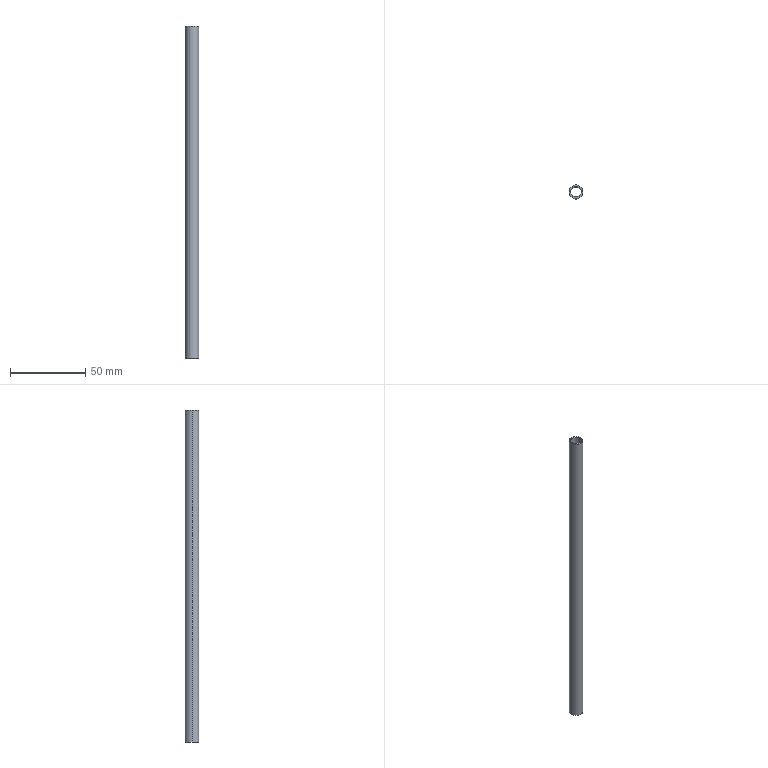Part | STEP file | DCV-000-018 | 1 solid | 6 faces | box 9 x 9 x 220 mm | volume 5529 mm3 | cylinder 4 | plane 2 | commonest cylinder face diameters 7 x2 9 x2
STEP:
#1=CARTESIAN_POINT('',(0.,0.,0.));
#2=DIRECTION('',(0.,0.,1.));
#3=DIRECTION('',(1.,0.,0.));
#4=AXIS2_PLACEMENT_3D('',#1,#2,#3);
#5=CARTESIAN_POINT('',(-3.5,0.,0.));
#6=VERTEX_POINT('',#5);
#7=CARTESIAN_POINT('',(-3.5,0.,220.));
#8=VERTEX_POINT('',#7);
#9=CARTESIAN_POINT('',(-3.5,0.,0.));
#10=DIRECTION('',(0.,0.,1.));
#11=VECTOR('',#10,1.);
#12=LINE('',#9,#11);
#13=CARTESIAN_POINT('',(0.,0.,0.));
#14=DIRECTION('',(0.,0.,1.));
#15=DIRECTION('',(-1.,0.,0.));
#16=AXIS2_PLACEMENT_3D('',#13,#14,#15);
#17=CYLINDRICAL_SURFACE('',#16,3.5);
#18=CARTESIAN_POINT('',(6.283,0.));
#19=DIRECTION('',(0.,1.));
#20=VECTOR('',#19,1.);
#21=LINE('',#18,#20);
#22=(GEOMETRIC_REPRESENTATION_CONTEXT(2)PARAMETRIC_REPRESENTATION_CONTEXT()REPRESENTATION_CONTEXT('',''));
#23=DEFINITIONAL_REPRESENTATION('',(#21),#22);
#24=PCURVE('',#17,#23);
#25=CARTESIAN_POINT('',(0.,0.,0.));
#26=DIRECTION('',(0.,0.,1.));
#27=DIRECTION('',(-1.,0.,0.));
#28=AXIS2_PLACEMENT_3D('',#25,#26,#27);
#29=CYLINDRICAL_SURFACE('',#28,3.5);
#30=CARTESIAN_POINT('',(0.,0.));
#31=DIRECTION('',(0.,1.));
#32=VECTOR('',#31,1.);
#33=LINE('',#30,#32);
#34=(GEOMETRIC_REPRESENTATION_CONTEXT(2)PARAMETRIC_REPRESENTATION_CONTEXT()REPRESENTATION_CONTEXT('',''));
#35=DEFINITIONAL_REPRESENTATION('',(#33),#34);
#36=PCURVE('',#29,#35);
#37=SURFACE_CURVE('',#12,(#24,#36),.PCURVE_S1.);
#38=EDGE_CURVE('',#6,#8,#37,.T.);
#39=ORIENTED_EDGE('',*,*,#38,.T.);
#40=CARTESIAN_POINT('',(3.5,0.,220.));
#41=VERTEX_POINT('',#40);
#42=CARTESIAN_POINT('',(0.,0.,220.));
#43=DIRECTION('',(0.,0.,-1.));
#44=DIRECTION('',(-1.,0.,0.));
#45=AXIS2_PLACEMENT_3D('',#42,#43,#44);
#46=CIRCLE('',#45,3.5);
#47=CARTESIAN_POINT('',(6.283,220.));
#48=DIRECTION('',(-1.,0.));
#49=VECTOR('',#48,1.);
#50=LINE('',#47,#49);
#51=(GEOMETRIC_REPRESENTATION_CONTEXT(2)PARAMETRIC_REPRESENTATION_CONTEXT()REPRESENTATION_CONTEXT('',''));
#52=DEFINITIONAL_REPRESENTATION('',(#50),#51);
#53=PCURVE('',#17,#52);
#54=CARTESIAN_POINT('',(0.,0.,220.));
#55=DIRECTION('',(0.,0.,1.));
#56=DIRECTION('',(1.,0.,0.));
#57=AXIS2_PLACEMENT_3D('',#54,#55,#56);
#58=PLANE('',#57);
#59=CARTESIAN_POINT('',(-3.5,0.));
#60=CARTESIAN_POINT('',(-3.5,6.062));
#61=CARTESIAN_POINT('',(1.75,3.031));
#62=CARTESIAN_POINT('',(7.,0.));
#63=CARTESIAN_POINT('',(1.75,-3.031));
#64=CARTESIAN_POINT('',(-3.5,-6.062));
#65=CARTESIAN_POINT('',(-3.5,0.));
#66=(BOUNDED_CURVE()B_SPLINE_CURVE(2,(#59,#60,#61,#62,#63,#64,#65),.UNSPECIFIED.,.T.,.F.)B_SPLINE_CURVE_WITH_KNOTS((1,2,2,2,2,1),(-2.094,0.,2.094,4.189,6.283,8.378),.UNSPECIFIED.)CURVE()GEOMETRIC_REPRESENTATION_ITEM()RATIONAL_B_SPLINE_CURVE((1.,0.5,1.,0.5,1.,0.5,1.))REPRESENTATION_ITEM(''));
#67=(GEOMETRIC_REPRESENTATION_CONTEXT(2)PARAMETRIC_REPRESENTATION_CONTEXT()REPRESENTATION_CONTEXT('',''));
#68=DEFINITIONAL_REPRESENTATION('',(#66),#67);
#69=PCURVE('',#58,#68);
#70=SURFACE_CURVE('',#46,(#53,#69),.PCURVE_S1.);
#71=EDGE_CURVE('',#8,#41,#70,.T.);
#72=ORIENTED_EDGE('',*,*,#71,.T.);
#73=CARTESIAN_POINT('',(3.5,0.,0.));
#74=VERTEX_POINT('',#73);
#75=CARTESIAN_POINT('',(3.5,0.,0.));
#76=DIRECTION('',(0.,0.,1.));
#77=VECTOR('',#76,1.);
#78=LINE('',#75,#77);
#79=CARTESIAN_POINT('',(3.142,0.));
#80=DIRECTION('',(0.,1.));
#81=VECTOR('',#80,1.);
#82=LINE('',#79,#81);
#83=(GEOMETRIC_REPRESENTATION_CONTEXT(2)PARAMETRIC_REPRESENTATION_CONTEXT()REPRESENTATION_CONTEXT('',''));
#84=DEFINITIONAL_REPRESENTATION('',(#82),#83);
#85=PCURVE('',#17,#84);
#86=CARTESIAN_POINT('',(3.142,0.));
#87=DIRECTION('',(0.,1.));
#88=VECTOR('',#87,1.);
#89=LINE('',#86,#88);
#90=(GEOMETRIC_REPRESENTATION_CONTEXT(2)PARAMETRIC_REPRESENTATION_CONTEXT()REPRESENTATION_CONTEXT('',''));
#91=DEFINITIONAL_REPRESENTATION('',(#89),#90);
#92=PCURVE('',#29,#91);
#93=SURFACE_CURVE('',#78,(#85,#92),.PCURVE_S1.);
#94=EDGE_CURVE('',#74,#41,#93,.T.);
#95=ORIENTED_EDGE('',*,*,#94,.F.);
#96=CARTESIAN_POINT('',(0.,0.,0.));
#97=DIRECTION('',(0.,0.,-1.));
#98=DIRECTION('',(-1.,0.,0.));
#99=AXIS2_PLACEMENT_3D('',#96,#97,#98);
#100=CIRCLE('',#99,3.5);
#101=CARTESIAN_POINT('',(6.283,0.));
#102=DIRECTION('',(-1.,0.));
#103=VECTOR('',#102,1.);
#104=LINE('',#101,#103);
#105=(GEOMETRIC_REPRESENTATION_CONTEXT(2)PARAMETRIC_REPRESENTATION_CONTEXT()REPRESENTATION_CONTEXT('',''));
#106=DEFINITIONAL_REPRESENTATION('',(#104),#105);
#107=PCURVE('',#17,#106);
#108=CARTESIAN_POINT('',(0.,0.,0.));
#109=DIRECTION('',(0.,0.,1.));
#110=DIRECTION('',(1.,0.,0.));
#111=AXIS2_PLACEMENT_3D('',#108,#109,#110);
#112=PLANE('',#111);
#113=CARTESIAN_POINT('',(-3.5,0.));
#114=CARTESIAN_POINT('',(-3.5,6.062));
#115=CARTESIAN_POINT('',(1.75,3.031));
#116=CARTESIAN_POINT('',(7.,0.));
#117=CARTESIAN_POINT('',(1.75,-3.031));
#118=CARTESIAN_POINT('',(-3.5,-6.062));
#119=CARTESIAN_POINT('',(-3.5,0.));
#120=(BOUNDED_CURVE()B_SPLINE_CURVE(2,(#113,#114,#115,#116,#117,#118,#119),.UNSPECIFIED.,.T.,.F.)B_SPLINE_CURVE_WITH_KNOTS((1,2,2,2,2,1),(-2.094,0.,2.094,4.189,6.283,8.378),.UNSPECIFIED.)CURVE()GEOMETRIC_REPRESENTATION_ITEM()RATIONAL_B_SPLINE_CURVE((1.,0.5,1.,0.5,1.,0.5,1.))REPRESENTATION_ITEM(''));
#121=(GEOMETRIC_REPRESENTATION_CONTEXT(2)PARAMETRIC_REPRESENTATION_CONTEXT()REPRESENTATION_CONTEXT('',''));
#122=DEFINITIONAL_REPRESENTATION('',(#120),#121);
#123=PCURVE('',#112,#122);
#124=SURFACE_CURVE('',#100,(#107,#123),.PCURVE_S1.);
#125=EDGE_CURVE('',#6,#74,#124,.T.);
#126=ORIENTED_EDGE('',*,*,#125,.F.);
#127=EDGE_LOOP('',(#39,#72,#95,#126));
#128=FACE_BOUND('',#127,.F.);
#129=ADVANCED_FACE('',(#128),#17,.F.);
#130=CARTESIAN_POINT('',(4.5,0.,0.));
#131=VERTEX_POINT('',#130);
#132=CARTESIAN_POINT('',(-4.5,0.,0.));
#133=VERTEX_POINT('',#132);
#134=CARTESIAN_POINT('',(0.,0.,0.));
#135=DIRECTION('',(0.,0.,1.));
#136=DIRECTION('',(1.,0.,0.));
#137=AXIS2_PLACEMENT_3D('',#134,#135,#136);
#138=CIRCLE('',#137,4.5);
#139=CARTESIAN_POINT('',(0.,0.,0.));
#140=DIRECTION('',(0.,0.,1.));
#141=DIRECTION('',(1.,0.,0.));
#142=AXIS2_PLACEMENT_3D('',#139,#140,#141);
#143=CYLINDRICAL_SURFACE('',#142,4.5);
#144=CARTESIAN_POINT('',(0.,0.));
#145=DIRECTION('',(1.,0.));
#146=VECTOR('',#145,1.);
#147=LINE('',#144,#146);
#148=(GEOMETRIC_REPRESENTATION_CONTEXT(2)PARAMETRIC_REPRESENTATION_CONTEXT()REPRESENTATION_CONTEXT('',''));
#149=DEFINITIONAL_REPRESENTATION('',(#147),#148);
#150=PCURVE('',#143,#149);
#151=CARTESIAN_POINT('',(0.,0.));
#152=DIRECTION('',(1.,0.));
#153=AXIS2_PLACEMENT_2D('',#151,#152);
#154=CIRCLE('',#153,4.5);
#155=(GEOMETRIC_REPRESENTATION_CONTEXT(2)PARAMETRIC_REPRESENTATION_CONTEXT()REPRESENTATION_CONTEXT('',''));
#156=DEFINITIONAL_REPRESENTATION('',(#154),#155);
#157=PCURVE('',#112,#156);
#158=SURFACE_CURVE('',#138,(#150,#157),.PCURVE_S1.);
#159=EDGE_CURVE('',#131,#133,#158,.T.);
#160=ORIENTED_EDGE('',*,*,#159,.T.);
#161=CARTESIAN_POINT('',(-4.5,0.,220.));
#162=VERTEX_POINT('',#161);
#163=CARTESIAN_POINT('',(-4.5,0.,0.));
#164=DIRECTION('',(0.,0.,1.));
#165=VECTOR('',#164,1.);
#166=LINE('',#163,#165);
#167=CARTESIAN_POINT('',(3.142,0.));
#168=DIRECTION('',(0.,1.));
#169=VECTOR('',#168,1.);
#170=LINE('',#167,#169);
#171=(GEOMETRIC_REPRESENTATION_CONTEXT(2)PARAMETRIC_REPRESENTATION_CONTEXT()REPRESENTATION_CONTEXT('',''));
#172=DEFINITIONAL_REPRESENTATION('',(#170),#171);
#173=PCURVE('',#143,#172);
#174=CARTESIAN_POINT('',(0.,0.,0.));
#175=DIRECTION('',(0.,0.,1.));
#176=DIRECTION('',(1.,0.,0.));
#177=AXIS2_PLACEMENT_3D('',#174,#175,#176);
#178=CYLINDRICAL_SURFACE('',#177,4.5);
#179=CARTESIAN_POINT('',(3.142,0.));
#180=DIRECTION('',(0.,1.));
#181=VECTOR('',#180,1.);
#182=LINE('',#179,#181);
#183=(GEOMETRIC_REPRESENTATION_CONTEXT(2)PARAMETRIC_REPRESENTATION_CONTEXT()REPRESENTATION_CONTEXT('',''));
#184=DEFINITIONAL_REPRESENTATION('',(#182),#183);
#185=PCURVE('',#178,#184);
#186=SURFACE_CURVE('',#166,(#173,#185),.PCURVE_S1.);
#187=EDGE_CURVE('',#133,#162,#186,.T.);
#188=ORIENTED_EDGE('',*,*,#187,.T.);
#189=CARTESIAN_POINT('',(4.5,0.,220.));
#190=VERTEX_POINT('',#189);
#191=CARTESIAN_POINT('',(0.,0.,220.));
#192=DIRECTION('',(0.,0.,1.));
#193=DIRECTION('',(1.,0.,0.));
#194=AXIS2_PLACEMENT_3D('',#191,#192,#193);
#195=CIRCLE('',#194,4.5);
#196=CARTESIAN_POINT('',(0.,220.));
#197=DIRECTION('',(1.,0.));
#198=VECTOR('',#197,1.);
#199=LINE('',#196,#198);
#200=(GEOMETRIC_REPRESENTATION_CONTEXT(2)PARAMETRIC_REPRESENTATION_CONTEXT()REPRESENTATION_CONTEXT('',''));
#201=DEFINITIONAL_REPRESENTATION('',(#199),#200);
#202=PCURVE('',#143,#201);
#203=CARTESIAN_POINT('',(0.,0.));
#204=DIRECTION('',(1.,0.));
#205=AXIS2_PLACEMENT_2D('',#203,#204);
#206=CIRCLE('',#205,4.5);
#207=(GEOMETRIC_REPRESENTATION_CONTEXT(2)PARAMETRIC_REPRESENTATION_CONTEXT()REPRESENTATION_CONTEXT('',''));
#208=DEFINITIONAL_REPRESENTATION('',(#206),#207);
#209=PCURVE('',#58,#208);
#210=SURFACE_CURVE('',#195,(#202,#209),.PCURVE_S1.);
#211=EDGE_CURVE('',#190,#162,#210,.T.);
#212=ORIENTED_EDGE('',*,*,#211,.F.);
#213=CARTESIAN_POINT('',(4.5,0.,0.));
#214=DIRECTION('',(0.,0.,1.));
#215=VECTOR('',#214,1.);
#216=LINE('',#213,#215);
#217=CARTESIAN_POINT('',(0.,0.));
#218=DIRECTION('',(0.,1.));
#219=VECTOR('',#218,1.);
#220=LINE('',#217,#219);
#221=(GEOMETRIC_REPRESENTATION_CONTEXT(2)PARAMETRIC_REPRESENTATION_CONTEXT()REPRESENTATION_CONTEXT('',''));
#222=DEFINITIONAL_REPRESENTATION('',(#220),#221);
#223=PCURVE('',#143,#222);
#224=CARTESIAN_POINT('',(6.283,0.));
#225=DIRECTION('',(0.,1.));
#226=VECTOR('',#225,1.);
#227=LINE('',#224,#226);
#228=(GEOMETRIC_REPRESENTATION_CONTEXT(2)PARAMETRIC_REPRESENTATION_CONTEXT()REPRESENTATION_CONTEXT('',''));
#229=DEFINITIONAL_REPRESENTATION('',(#227),#228);
#230=PCURVE('',#178,#229);
#231=SURFACE_CURVE('',#216,(#223,#230),.PCURVE_S1.);
#232=EDGE_CURVE('',#131,#190,#231,.T.);
#233=ORIENTED_EDGE('',*,*,#232,.F.);
#234=EDGE_LOOP('',(#160,#188,#212,#233));
#235=FACE_BOUND('',#234,.T.);
#236=ADVANCED_FACE('',(#235),#143,.T.);
#237=ORIENTED_EDGE('',*,*,#125,.F.);
#238=CARTESIAN_POINT('',(0.,0.,0.));
#239=DIRECTION('',(0.,0.,-1.));
#240=DIRECTION('',(-1.,0.,0.));
#241=AXIS2_PLACEMENT_3D('',#238,#239,#240);
#242=CIRCLE('',#241,3.5);
#243=CARTESIAN_POINT('',(-3.5,0.));
#244=CARTESIAN_POINT('',(-3.5,6.062));
#245=CARTESIAN_POINT('',(1.75,3.031));
#246=CARTESIAN_POINT('',(7.,0.));
#247=CARTESIAN_POINT('',(1.75,-3.031));
#248=CARTESIAN_POINT('',(-3.5,-6.062));
#249=CARTESIAN_POINT('',(-3.5,0.));
#250=(BOUNDED_CURVE()B_SPLINE_CURVE(2,(#243,#244,#245,#246,#247,#248,#249),.UNSPECIFIED.,.T.,.F.)B_SPLINE_CURVE_WITH_KNOTS((1,2,2,2,2,1),(-2.094,0.,2.094,4.189,6.283,8.378),.UNSPECIFIED.)CURVE()GEOMETRIC_REPRESENTATION_ITEM()RATIONAL_B_SPLINE_CURVE((1.,0.5,1.,0.5,1.,0.5,1.))REPRESENTATION_ITEM(''));
#251=(GEOMETRIC_REPRESENTATION_CONTEXT(2)PARAMETRIC_REPRESENTATION_CONTEXT()REPRESENTATION_CONTEXT('',''));
#252=DEFINITIONAL_REPRESENTATION('',(#250),#251);
#253=PCURVE('',#112,#252);
#254=CARTESIAN_POINT('',(6.283,0.));
#255=DIRECTION('',(-1.,0.));
#256=VECTOR('',#255,1.);
#257=LINE('',#254,#256);
#258=(GEOMETRIC_REPRESENTATION_CONTEXT(2)PARAMETRIC_REPRESENTATION_CONTEXT()REPRESENTATION_CONTEXT('',''));
#259=DEFINITIONAL_REPRESENTATION('',(#257),#258);
#260=PCURVE('',#29,#259);
#261=SURFACE_CURVE('',#242,(#253,#260),.PCURVE_S1.);
#262=EDGE_CURVE('',#74,#6,#261,.T.);
#263=ORIENTED_EDGE('',*,*,#262,.F.);
#264=EDGE_LOOP('',(#237,#263));
#265=FACE_BOUND('',#264,.T.);
#266=ORIENTED_EDGE('',*,*,#159,.F.);
#267=CARTESIAN_POINT('',(0.,0.,0.));
#268=DIRECTION('',(0.,0.,1.));
#269=DIRECTION('',(1.,0.,0.));
#270=AXIS2_PLACEMENT_3D('',#267,#268,#269);
#271=CIRCLE('',#270,4.5);
#272=CARTESIAN_POINT('',(0.,0.));
#273=DIRECTION('',(1.,0.));
#274=AXIS2_PLACEMENT_2D('',#272,#273);
#275=CIRCLE('',#274,4.5);
#276=(GEOMETRIC_REPRESENTATION_CONTEXT(2)PARAMETRIC_REPRESENTATION_CONTEXT()REPRESENTATION_CONTEXT('',''));
#277=DEFINITIONAL_REPRESENTATION('',(#275),#276);
#278=PCURVE('',#112,#277);
#279=CARTESIAN_POINT('',(0.,0.));
#280=DIRECTION('',(1.,0.));
#281=VECTOR('',#280,1.);
#282=LINE('',#279,#281);
#283=(GEOMETRIC_REPRESENTATION_CONTEXT(2)PARAMETRIC_REPRESENTATION_CONTEXT()REPRESENTATION_CONTEXT('',''));
#284=DEFINITIONAL_REPRESENTATION('',(#282),#283);
#285=PCURVE('',#178,#284);
#286=SURFACE_CURVE('',#271,(#278,#285),.PCURVE_S1.);
#287=EDGE_CURVE('',#133,#131,#286,.T.);
#288=ORIENTED_EDGE('',*,*,#287,.F.);
#289=EDGE_LOOP('',(#266,#288));
#290=FACE_BOUND('',#289,.T.);
#291=ADVANCED_FACE('',(#265,#290),#112,.F.);
#292=ORIENTED_EDGE('',*,*,#71,.T.);
#293=CARTESIAN_POINT('',(0.,0.,220.));
#294=DIRECTION('',(0.,0.,-1.));
#295=DIRECTION('',(-1.,0.,0.));
#296=AXIS2_PLACEMENT_3D('',#293,#294,#295);
#297=CIRCLE('',#296,3.5);
#298=CARTESIAN_POINT('',(-3.5,0.));
#299=CARTESIAN_POINT('',(-3.5,6.062));
#300=CARTESIAN_POINT('',(1.75,3.031));
#301=CARTESIAN_POINT('',(7.,0.));
#302=CARTESIAN_POINT('',(1.75,-3.031));
#303=CARTESIAN_POINT('',(-3.5,-6.062));
#304=CARTESIAN_POINT('',(-3.5,0.));
#305=(BOUNDED_CURVE()B_SPLINE_CURVE(2,(#298,#299,#300,#301,#302,#303,#304),.UNSPECIFIED.,.T.,.F.)B_SPLINE_CURVE_WITH_KNOTS((1,2,2,2,2,1),(-2.094,0.,2.094,4.189,6.283,8.378),.UNSPECIFIED.)CURVE()GEOMETRIC_REPRESENTATION_ITEM()RATIONAL_B_SPLINE_CURVE((1.,0.5,1.,0.5,1.,0.5,1.))REPRESENTATION_ITEM(''));
#306=(GEOMETRIC_REPRESENTATION_CONTEXT(2)PARAMETRIC_REPRESENTATION_CONTEXT()REPRESENTATION_CONTEXT('',''));
#307=DEFINITIONAL_REPRESENTATION('',(#305),#306);
#308=PCURVE('',#58,#307);
#309=CARTESIAN_POINT('',(6.283,220.));
#310=DIRECTION('',(-1.,0.));
#311=VECTOR('',#310,1.);
#312=LINE('',#309,#311);
#313=(GEOMETRIC_REPRESENTATION_CONTEXT(2)PARAMETRIC_REPRESENTATION_CONTEXT()REPRESENTATION_CONTEXT('',''));
#314=DEFINITIONAL_REPRESENTATION('',(#312),#313);
#315=PCURVE('',#29,#314);
#316=SURFACE_CURVE('',#297,(#308,#315),.PCURVE_S1.);
#317=EDGE_CURVE('',#41,#8,#316,.T.);
#318=ORIENTED_EDGE('',*,*,#317,.T.);
#319=EDGE_LOOP('',(#292,#318));
#320=FACE_BOUND('',#319,.T.);
#321=ORIENTED_EDGE('',*,*,#211,.T.);
#322=CARTESIAN_POINT('',(0.,0.,220.));
#323=DIRECTION('',(0.,0.,1.));
#324=DIRECTION('',(1.,0.,0.));
#325=AXIS2_PLACEMENT_3D('',#322,#323,#324);
#326=CIRCLE('',#325,4.5);
#327=CARTESIAN_POINT('',(0.,0.));
#328=DIRECTION('',(1.,0.));
#329=AXIS2_PLACEMENT_2D('',#327,#328);
#330=CIRCLE('',#329,4.5);
#331=(GEOMETRIC_REPRESENTATION_CONTEXT(2)PARAMETRIC_REPRESENTATION_CONTEXT()REPRESENTATION_CONTEXT('',''));
#332=DEFINITIONAL_REPRESENTATION('',(#330),#331);
#333=PCURVE('',#58,#332);
#334=CARTESIAN_POINT('',(0.,220.));
#335=DIRECTION('',(1.,0.));
#336=VECTOR('',#335,1.);
#337=LINE('',#334,#336);
#338=(GEOMETRIC_REPRESENTATION_CONTEXT(2)PARAMETRIC_REPRESENTATION_CONTEXT()REPRESENTATION_CONTEXT('',''));
#339=DEFINITIONAL_REPRESENTATION('',(#337),#338);
#340=PCURVE('',#178,#339);
#341=SURFACE_CURVE('',#326,(#333,#340),.PCURVE_S1.);
#342=EDGE_CURVE('',#162,#190,#341,.T.);
#343=ORIENTED_EDGE('',*,*,#342,.T.);
#344=EDGE_LOOP('',(#321,#343));
#345=FACE_BOUND('',#344,.T.);
#346=ADVANCED_FACE('',(#320,#345),#58,.T.);
#347=ORIENTED_EDGE('',*,*,#187,.F.);
#348=ORIENTED_EDGE('',*,*,#287,.T.);
#349=ORIENTED_EDGE('',*,*,#232,.T.);
#350=ORIENTED_EDGE('',*,*,#342,.F.);
#351=EDGE_LOOP('',(#347,#348,#349,#350));
#352=FACE_BOUND('',#351,.T.);
#353=ADVANCED_FACE('',(#352),#178,.T.);
#354=ORIENTED_EDGE('',*,*,#317,.T.);
#355=ORIENTED_EDGE('',*,*,#38,.F.);
#356=ORIENTED_EDGE('',*,*,#262,.F.);
#357=ORIENTED_EDGE('',*,*,#94,.T.);
#358=EDGE_LOOP('',(#354,#355,#356,#357));
#359=FACE_BOUND('',#358,.F.);
#360=ADVANCED_FACE('',(#359),#29,.F.);
#361=CLOSED_SHELL('',(#129,#236,#291,#346,#353,#360));
#362=MANIFOLD_SOLID_BREP('',#361);
#363=(LENGTH_UNIT()NAMED_UNIT(*)SI_UNIT(.MILLI.,.METRE.));
#364=UNCERTAINTY_MEASURE_WITH_UNIT(LENGTH_MEASURE(0.0000001),#363,'','');
#365=(NAMED_UNIT(*)PLANE_ANGLE_UNIT()SI_UNIT($,.RADIAN.));
#366=(NAMED_UNIT(*)SI_UNIT($,.STERADIAN.)SOLID_ANGLE_UNIT());
#367=(GEOMETRIC_REPRESENTATION_CONTEXT(3)GLOBAL_UNCERTAINTY_ASSIGNED_CONTEXT((#364))GLOBAL_UNIT_ASSIGNED_CONTEXT((#363,#365,#366))REPRESENTATION_CONTEXT('',''));
#368=ADVANCED_BREP_SHAPE_REPRESENTATION('',(#4,#362),#367);